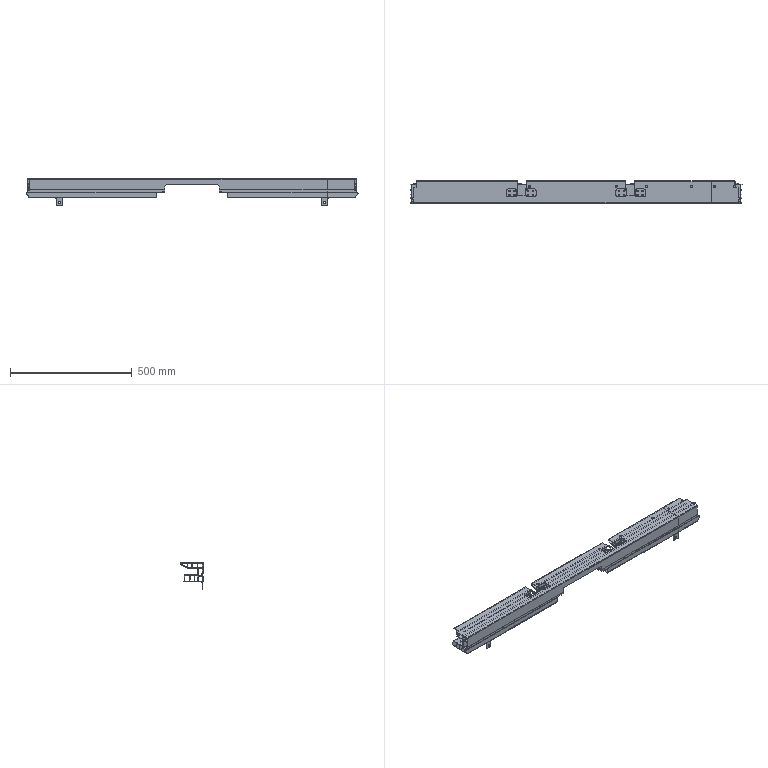NC program | NX | posted with a generic post | part box 1365 x 90.95 x 108.501 mm
Lines 36 to 1103 of 25066:
(CAVITY_MILL_1 , TOOL : D16)
N64 T16 M6
N66 G54
N68 G17 G0 G90 X693.761 Y-28.858 B0. C0. S9500 M3
N70 G43 Z30. H16
N72 Z0.527
N74 G94 G1 Z-0.973 F1000.
N76 X683.861 Y-34.573
N78 G3 X683.361 Y-35.439 R1.
N80 G1 X676.161
N82 Y-31.805 F2500.
N84 G2 X672.3 Y-33.633 R15.3
N86 G1 Y-39.073
N88 X676.161
N90 Y-35.439
N92 X683.361
N94 Y17.129
N96 G3 X684.77 Y22.775 R12.02
N98 G1 Y24.556
N100 G3 X683.361 Y30.203 R12.02
N102 G1 Y45.471
N104 G3 X682.561 Y46.273 R0.802
N106 G1 X677.738
N108 G3 X673.784 Y53.473 R10.019
N110 G1 X669.02
N112 G2 X675.85 Y45.473 R8.099
N114 G1 Y34.505
N116 X675.963 Y34.436
N118 X678.059 Y33.148
N120 G2 X682.85 Y24.556 R10.1
N122 G1 Y22.775
N124 G2 X675.85 Y13.163 R10.1
N126 G1 Y-19.025
N128 G2 X667.75 Y-27.125 R8.1
N130 G1 X665.1
N132 Y-45.473
N134 G2 X658.27 Y-53.473 R8.1
N136 G1 X663.033
N138 G3 X666.988 Y-46.273 R10.02
N140 G1 X682.561
N142 G3 X683.361 Y-45.473 R0.8
N144 G1 Y-35.439
N146 G2 X683.861 Y-34.573 R1.
N148 G1 X693.761 Y-28.858
N150 Z0.527
N152 G0 Z-0.444
N154 G1 Z-1.944 F1000.
N156 X683.861 Y-34.574
N158 G3 X683.361 Y-35.44 R1.
N160 G1 X676.161
N162 Y-31.805 F2500.
N164 G2 X672.3 Y-33.633 R15.3
N166 G1 Y-39.075
N168 X676.161
N170 Y-35.44
N172 X683.361
N174 Y17.129
N176 G3 X684.77 Y22.775 R12.02
N178 G1 Y24.556
N180 G3 X683.361 Y30.203 R12.02
N182 G1 Y45.475
N184 G3 X682.561 Y46.275 R0.8
N186 G1 X677.738
N188 G3 X673.783 Y53.475 R10.02
N190 G1 X669.019
N192 G2 X675.85 Y45.475 R8.1
N194 G1 Y34.505
N196 X675.933 Y34.455
N198 X678.059 Y33.148
N200 G2 X682.85 Y24.556 R10.1
N202 G1 Y22.775
N204 G2 X675.85 Y13.163 R10.1
N206 G1 Y-19.025
N208 G2 X667.75 Y-27.125 R8.1
N210 G1 X665.1
N212 Y-45.475
N214 G2 X658.269 Y-53.475 R8.1
N216 G1 X663.033
N218 G3 X666.988 Y-46.275 R10.02
N220 G1 X682.561
N222 G3 X683.361 Y-45.475 R0.8
N224 G1 Y-35.44
N226 G2 X683.861 Y-34.574 R1.
N228 G1 X693.761 Y-28.858
N230 Z-0.444
N232 G0 Z-1.416
N234 G1 Z-2.916 F1000.
N236 X683.861 Y-34.574
N238 G3 X683.361 Y-35.44 R1.
N240 G1 X676.161
N242 Y-31.805 F2500.
N244 G2 X672.3 Y-33.633 R15.3
N246 G1 Y-39.075
N248 X676.161
N250 Y-35.44
N252 X683.361
N254 Y17.129
N256 G3 X684.77 Y22.775 R12.02
N258 G1 Y24.556
N260 G3 X683.361 Y30.203 R12.02
N262 G1 Y45.475
N264 G3 X682.561 Y46.275 R0.8
N266 G1 X677.738
N268 G3 X673.783 Y53.475 R10.02
N270 G1 X669.019
N272 G2 X675.85 Y45.475 R8.1
N274 G1 Y34.505
N276 X675.963 Y34.436
N278 X678.059 Y33.148
N280 G2 X682.85 Y24.556 R10.1
N282 G1 Y22.775
N284 G2 X675.85 Y13.163 R10.1
N286 G1 Y-19.025
N288 G2 X667.75 Y-27.125 R8.1
N290 G1 X665.1
N292 Y-45.475
N294 G2 X658.269 Y-53.475 R8.1
N296 G1 X663.033
N298 G3 X666.988 Y-46.275 R10.02
N300 G1 X682.561
N302 G3 X683.361 Y-45.475 R0.8
N304 G1 Y-35.44
N306 G2 X683.861 Y-34.574 R1.
N308 G1 X693.761 Y-28.858
N310 Z-1.416
N312 G0 Z-2.387
N314 G1 Z-3.887 F1000.
N316 X683.861 Y-34.574
N318 G3 X683.361 Y-35.44 R1.
N320 G1 X676.161
N322 Y-31.805 F2500.
N324 G2 X672.3 Y-33.633 R15.3
N326 G1 Y-39.075
N328 X676.161
N330 Y-35.44
N332 X683.361
N334 Y17.129
N336 G3 X684.77 Y22.775 R12.02
N338 G1 Y24.556
N340 G3 X683.361 Y30.203 R12.02
N342 G1 Y45.475
N344 G3 X682.561 Y46.275 R0.8
N346 G1 X677.738
N348 G3 X673.783 Y53.475 R10.02
N350 G1 X669.019
N352 G2 X675.85 Y45.475 R8.1
N354 G1 Y34.505
N356 X675.963 Y34.436
N358 X678.059 Y33.148
N360 G2 X682.85 Y24.556 R10.1
N362 G1 Y22.775
N364 G2 X675.85 Y13.163 R10.1
N366 G1 Y-19.025
N368 G2 X667.75 Y-27.125 R8.1
N370 G1 X665.1
N372 Y-45.475
N374 G2 X658.269 Y-53.475 R8.1
N376 G1 X663.033
N378 G3 X666.988 Y-46.275 R10.02
N380 G1 X682.561
N382 G3 X683.361 Y-45.475 R0.8
N384 G1 Y-35.44
N386 G2 X683.861 Y-34.574 R1.
N388 G1 X693.761 Y-28.858
N390 Z-2.387
N392 G0 Z-3.358
N394 G1 Z-4.858 F1000.
N396 X683.861 Y-34.574
N398 G3 X683.361 Y-35.44 R1.
N400 G1 X676.161
N402 Y-31.805 F2500.
N404 G2 X672.3 Y-33.633 R15.3
N406 G1 Y-39.075
N408 X676.161
N410 Y-35.44
N412 X683.361
N414 Y17.129
N416 G3 X684.77 Y22.775 R12.02
N418 G1 Y24.556
N420 G3 X683.361 Y30.203 R12.02
N422 G1 Y45.475
N424 G3 X682.561 Y46.275 R0.8
N426 G1 X677.738
N428 G3 X673.783 Y53.475 R10.02
N430 G1 X669.019
N432 G2 X675.85 Y45.475 R8.1
N434 G1 Y34.505
N436 X675.963 Y34.436
N438 X678.059 Y33.148
N440 G2 X682.85 Y24.556 R10.1
N442 G1 Y22.775
N444 G2 X675.85 Y13.163 R10.1
N446 G1 Y-19.025
N448 G2 X667.75 Y-27.125 R8.1
N450 G1 X665.1
N452 Y-45.475
N454 G2 X658.269 Y-53.475 R8.1
N456 G1 X663.033
N458 G3 X666.988 Y-46.275 R10.02
N460 G1 X682.561
N462 G3 X683.361 Y-45.475 R0.8
N464 G1 Y-35.44
N466 G2 X683.861 Y-34.574 R1.
N468 G1 X693.761 Y-28.858
N470 Z-3.358
N472 G0 Z-4.33
N474 G1 Z-5.83 F1000.
N476 X683.861 Y-34.574
N478 G3 X683.361 Y-35.44 R1.
N480 G1 X676.161
N482 Y-31.805 F2500.
N484 G2 X672.3 Y-33.633 R15.3
N486 G1 Y-39.075
N488 X676.161
N490 Y-35.44
N492 X683.361
N494 Y17.129
N496 G3 X684.77 Y22.775 R12.02
N498 G1 Y24.556
N500 G3 X683.361 Y30.203 R12.02
N502 G1 Y45.475
N504 G3 X682.561 Y46.275 R0.8
N506 G1 X677.738
N508 G3 X673.783 Y53.475 R10.02
N510 G1 X669.019
N512 G2 X675.85 Y45.475 R8.1
N514 G1 Y34.505
N516 X678.059 Y33.148
N518 G2 X682.85 Y24.556 R10.1
N520 G1 Y22.775
N522 G2 X675.85 Y13.163 R10.1
N524 G1 Y-19.025
N526 G2 X667.75 Y-27.125 R8.1
N528 G1 X665.1
N530 Y-45.475
N532 G2 X658.269 Y-53.475 R8.1
N534 G1 X663.033
N536 G3 X666.988 Y-46.275 R10.02
N538 G1 X682.561
N540 G3 X683.361 Y-45.475 R0.8
N542 G1 Y-35.44
N544 G2 X683.861 Y-34.574 R1.
N546 G1 X693.761 Y-28.858
N548 Z-4.33
N550 G0 Z-5.301
N552 G1 Z-6.801 F1000.
N554 X683.861 Y-34.574
N556 G3 X683.361 Y-35.44 R1.
N558 G1 X676.161
N560 Y-31.805 F2500.
N562 G2 X672.3 Y-33.633 R15.3
N564 G1 Y-39.075
N566 X676.161
N568 Y-35.44
N570 X683.361
N572 Y17.129
N574 G3 X684.77 Y22.775 R12.02
N576 G1 Y24.556
N578 G3 X683.361 Y30.203 R12.02
N580 G1 Y45.475
N582 G3 X682.561 Y46.275 R0.8
N584 G1 X677.738
N586 G3 X673.783 Y53.475 R10.02
N588 G1 X669.019
N590 G2 X675.85 Y45.475 R8.1
N592 G1 Y34.505
N594 X678.059 Y33.148
N596 G2 X682.85 Y24.556 R10.1
N598 G1 Y22.775
N600 G2 X675.85 Y13.163 R10.1
N602 G1 Y-19.025
N604 G2 X667.75 Y-27.125 R8.1
N606 G1 X665.1
N608 Y-45.475
N610 G2 X658.269 Y-53.475 R8.1
N612 G1 X663.033
N614 G3 X666.988 Y-46.275 R10.02
N616 G1 X682.561
N618 G3 X683.361 Y-45.475 R0.8
N620 G1 Y-35.44
N622 G2 X683.861 Y-34.574 R1.
N624 G1 X693.761 Y-28.858
N626 Z-5.301
N628 G0 Z-6.273
N630 G1 Z-7.773 F1000.
N632 X683.861 Y-34.574
N634 G3 X683.361 Y-35.44 R1.
N636 G1 X676.161
N638 Y-31.805 F2500.
N640 G2 X672.3 Y-33.633 R15.3
N642 G1 Y-39.075
N644 X676.161
N646 Y-35.44
N648 X683.361
N650 Y17.129
N652 G3 X684.77 Y22.775 R12.02
N654 G1 Y24.556
N656 G3 X683.361 Y30.203 R12.02
N658 G1 Y45.475
N660 G3 X682.561 Y46.275 R0.8
N662 G1 X677.738
N664 G3 X673.783 Y53.475 R10.02
N666 G1 X669.019
N668 G2 X675.85 Y45.475 R8.1
N670 G1 Y34.505
N672 X678.059 Y33.148
N674 G2 X682.85 Y24.556 R10.1
N676 G1 Y22.775
N678 G2 X675.85 Y13.163 R10.1
N680 G1 Y-19.025
N682 G2 X667.75 Y-27.125 R8.1
N684 G1 X665.1
N686 Y-45.475
N688 G2 X658.269 Y-53.475 R8.1
N690 G1 X663.033
N692 G3 X666.988 Y-46.275 R10.02
N694 G1 X682.561
N696 G3 X683.361 Y-45.475 R0.8
N698 G1 Y-35.44
N700 G2 X683.861 Y-34.574 R1.
N702 G1 X693.761 Y-28.858
N704 Z-6.273
N706 G0 Z-7.244
N708 G1 Z-8.744 F1000.
N710 X683.861 Y-34.574
N712 G3 X683.361 Y-35.44 R1.
N714 G1 X676.161
N716 Y-31.805 F2500.
N718 G2 X672.3 Y-33.633 R15.3
N720 G1 Y-39.075
N722 X676.161
N724 Y-35.44
N726 X683.361
N728 Y17.129
N730 G3 X684.77 Y22.775 R12.02
N732 G1 Y24.556
N734 G3 X683.361 Y30.203 R12.02
N736 G1 Y45.475
N738 G3 X682.561 Y46.275 R0.8
N740 G1 X677.738
N742 G3 X673.783 Y53.475 R10.02
N744 G1 X669.019
N746 G2 X675.85 Y45.475 R8.1
N748 G1 Y34.505
N750 X678.059 Y33.148
N752 G2 X682.85 Y24.556 R10.1
N754 G1 Y22.775
N756 G2 X675.85 Y13.163 R10.1
N758 G1 Y-19.025
N760 G2 X667.75 Y-27.125 R8.1
N762 G1 X665.1
N764 Y-45.475
N766 G2 X658.269 Y-53.475 R8.1
N768 G1 X663.033
N770 G3 X666.988 Y-46.275 R10.02
N772 G1 X682.561
N774 G3 X683.361 Y-45.475 R0.8
N776 G1 Y-35.44
N778 G2 X683.861 Y-34.574 R1.
N780 G1 X693.761 Y-28.858
N782 Z-7.244
N784 G0 Z-8.216
N786 G1 Z-9.716 F1000.
N788 X683.861 Y-34.574
N790 G3 X683.361 Y-35.44 R1.
N792 G1 X676.161
N794 Y-31.805 F2500.
N796 G2 X672.3 Y-33.633 R15.3
N798 G1 Y-39.075
N800 X676.161
N802 Y-35.44
N804 X683.361
N806 Y17.129
N808 G3 X684.77 Y22.775 R12.02
N810 G1 Y24.556
N812 G3 X683.361 Y30.203 R12.02
N814 G1 Y45.475
N816 G3 X682.561 Y46.275 R0.8
N818 G1 X677.738
N820 G3 X673.783 Y53.475 R10.02
N822 G1 X669.019
N824 G2 X675.85 Y45.475 R8.1
N826 G1 Y34.505
N828 X678.059 Y33.149
N830 G2 X682.85 Y24.556 R10.1
N832 G1 Y22.775
N834 G2 X675.85 Y13.163 R10.1
N836 G1 Y-19.025
N838 G2 X667.75 Y-27.125 R8.1
N840 G1 X665.1
N842 Y-45.475
N844 G2 X658.269 Y-53.475 R8.1
N846 G1 X663.033
N848 G3 X666.988 Y-46.275 R10.02
N850 G1 X682.561
N852 G3 X683.361 Y-45.475 R0.8
N854 G1 Y-35.44
N856 G2 X683.861 Y-34.574 R1.
N858 G1 X693.761 Y-28.858
N860 Z-8.216
N862 G0 Z-9.187
N864 G1 Z-10.687 F1000.
N866 X683.861 Y-34.574
N868 G3 X683.361 Y-35.44 R1.
N870 G1 X676.161
N872 Y-31.805 F2500.
N874 G2 X672.3 Y-33.633 R15.3
N876 G1 Y-39.075
N878 X676.161
N880 Y-35.44
N882 X683.361
N884 Y17.129
N886 G3 X684.77 Y22.775 R12.02
N888 G1 Y24.556
N890 G3 X683.361 Y30.203 R12.02
N892 G1 Y45.475
N894 G3 X682.561 Y46.275 R0.8
N896 G1 X677.738
N898 G3 X673.783 Y53.475 R10.02
N900 G1 X669.019
N902 G2 X675.85 Y45.475 R8.1
N904 G1 Y34.505
N906 X678.037 Y33.162
N908 G2 X682.85 Y24.556 R10.1
N910 G1 Y22.775
N912 G2 X675.85 Y13.163 R10.1
N914 G1 Y-19.025
N916 G2 X667.75 Y-27.125 R8.1
N918 G1 X665.1
N920 Y-45.475
N922 G2 X658.269 Y-53.475 R8.1
N924 G1 X663.033
N926 G3 X666.988 Y-46.275 R10.02
N928 G1 X682.561
N930 G3 X683.361 Y-45.475 R0.8
N932 G1 Y-35.44
N934 G2 X683.861 Y-34.574 R1.
N936 G1 X693.761 Y-28.858
N938 Z-9.187
N940 G0 Z-10.158
N942 G1 Z-11.658 F1000.
N944 X683.861 Y-34.574
N946 G3 X683.361 Y-35.44 R1.
N948 G1 X676.161
N950 Y-31.805 F2500.
N952 G2 X672.3 Y-33.633 R15.3
N954 G1 Y-39.075
N956 X676.161
N958 Y-35.44
N960 X683.361
N962 Y17.129
N964 G3 X684.77 Y22.775 R12.02
N966 G1 Y24.556
N968 G3 X683.361 Y30.203 R12.02
N970 G1 Y45.475
N972 G3 X682.561 Y46.275 R0.8
N974 G1 X677.738
N976 G3 X673.783 Y53.475 R10.02
N978 G1 X669.019
N980 G2 X675.85 Y45.475 R8.1
N982 G1 Y34.505
N984 X678.037 Y33.162
N986 G2 X682.85 Y24.556 R10.1
N988 G1 Y22.775
N990 G2 X675.85 Y13.163 R10.1
N992 G1 Y-19.025
N994 G2 X667.75 Y-27.125 R8.1
N996 G1 X665.1
N998 Y-45.475
N1000 G2 X658.269 Y-53.475 R8.1
N1002 G1 X663.033
N1004 G3 X666.988 Y-46.275 R10.02
N1006 G1 X682.561
N1008 G3 X683.361 Y-45.475 R0.8
N1010 G1 Y-35.44
N1012 G2 X683.861 Y-34.574 R1.
N1014 G1 X693.761 Y-28.858
N1016 Z-10.158
N1018 G0 Z-11.13
N1020 G1 Z-12.63 F1000.
N1022 X683.861 Y-34.574
N1024 G3 X683.361 Y-35.44 R1.
N1026 G1 X676.161
N1028 Y-31.805 F2500.
N1030 G2 X672.3 Y-33.633 R15.3
N1032 G1 Y-39.075
N1034 X676.161
N1036 Y-35.44
N1038 X683.361
N1040 Y17.129
N1042 G3 X684.77 Y22.775 R12.02
N1044 G1 Y24.556
N1046 G3 X683.361 Y30.203 R12.02
N1048 G1 Y45.475
N1050 G3 X682.561 Y46.275 R0.8
N1052 G1 X677.738
N1054 G3 X673.783 Y53.475 R10.02
N1056 G1 X669.019
N1058 G2 X675.85 Y45.475 R8.1
N1060 G1 Y34.505
N1062 X678.037 Y33.162
N1064 G2 X682.85 Y24.556 R10.1
N1066 G1 Y22.775
N1068 G2 X675.85 Y13.163 R10.1
N1070 G1 Y-19.025
N1072 G2 X667.75 Y-27.125 R8.1
N1074 G1 X665.1
N1076 Y-45.475
N1078 G2 X658.269 Y-53.475 R8.1
N1080 G1 X663.033
N1082 G3 X666.988 Y-46.275 R10.02
N1084 G1 X682.561
N1086 G3 X683.361 Y-45.475 R0.8
N1088 G1 Y-35.44
N1090 G2 X683.861 Y-34.574 R1.
N1092 G1 X693.761 Y-28.858
N1094 Z-11.13
N1096 G0 Z-12.101
N1098 G1 Z-13.601 F1000.
N1100 X683.861 Y-34.574
N1102 G3 X683.361 Y-35.44 R1.
N1104 G1 X676.161
N1106 Y-31.805 F2500.
N1108 G2 X672.3 Y-33.633 R15.3
N1110 G1 Y-39.075
N1112 X676.161
N1114 Y-35.44
N1116 X683.361
N1118 Y17.129
N1120 G3 X684.77 Y22.775 R12.02
N1122 G1 Y24.556
N1124 G3 X683.361 Y30.203 R12.02
N1126 G1 Y45.475
N1128 G3 X682.561 Y46.275 R0.8
N1130 G1 X677.738
N1132 G3 X673.783 Y53.475 R10.02
N1134 G1 X669.019
N1136 G2 X675.85 Y45.475 R8.1
N1138 G1 Y34.505
N1140 X678.037 Y33.162
N1142 G2 X682.85 Y24.556 R10.1
N1144 G1 Y22.775
N1146 G2 X675.85 Y13.163 R10.1
N1148 G1 Y-19.025
N1150 G2 X667.75 Y-27.125 R8.1
N1152 G1 X665.1
N1154 Y-45.475
N1156 G2 X658.269 Y-53.475 R8.1
N1158 G1 X663.033
N1160 G3 X666.988 Y-46.275 R10.02
N1162 G1 X682.561
N1164 G3 X683.361 Y-45.475 R0.8
N1166 G1 Y-35.44
N1168 G2 X683.861 Y-34.574 R1.
N1170 G1 X693.761 Y-28.858
N1172 Z-12.101
N1174 G0 Z-13.073
N1176 G1 Z-14.573 F1000.
N1178 X683.861 Y-34.574
N1180 G3 X683.361 Y-35.44 R1.
N1182 G1 X676.161
N1184 Y-31.805 F2500.
N1186 G2 X672.3 Y-33.633 R15.3
N1188 G1 Y-39.075
N1190 X676.161
N1192 Y-35.44
N1194 X683.361
N1196 Y17.129
N1198 G3 X684.77 Y22.775 R12.02
N1200 G1 Y24.556
N1202 G3 X683.361 Y30.203 R12.02
N1204 G1 Y45.475
N1206 G3 X682.561 Y46.275 R0.8
N1208 G1 X677.738
N1210 G3 X673.783 Y53.475 R10.02
N1212 G1 X669.019
N1214 G2 X675.85 Y45.475 R8.1
N1216 G1 Y34.505
N1218 X678.037 Y33.162
N1220 G2 X682.85 Y24.556 R10.1
N1222 G1 Y22.775
N1224 G2 X675.85 Y13.163 R10.1
N1226 G1 Y-19.025
N1228 G2 X667.75 Y-27.125 R8.1
N1230 G1 X665.1
N1232 Y-45.475
N1234 G2 X658.269 Y-53.475 R8.1
N1236 G1 X663.033
N1238 G3 X666.988 Y-46.275 R10.02
N1240 G1 X682.561
N1242 G3 X683.361 Y-45.475 R0.8
N1244 G1 Y-35.44
N1246 G2 X683.861 Y-34.574 R1.
N1248 G1 X693.761 Y-28.858
N1250 Z-13.073
N1252 G0 Z-14.044
N1254 G1 Z-15.544 F1000.
N1256 X683.861 Y-34.574
N1258 G3 X683.361 Y-35.44 R1.
N1260 G1 X676.161
N1262 Y-31.805 F2500.
N1264 G2 X672.3 Y-33.633 R15.3
N1266 G1 Y-39.075
N1268 X676.161
N1270 Y-35.44
N1272 X683.361
N1274 Y17.129
N1276 G3 X684.77 Y22.775 R12.02
N1278 G1 Y24.556
N1280 G3 X683.361 Y30.203 R12.02
N1282 G1 Y45.475
N1284 G3 X682.561 Y46.275 R0.8
N1286 G1 X677.738
N1288 G3 X673.783 Y53.475 R10.02
N1290 G1 X669.019
N1292 G2 X675.85 Y45.475 R8.1
N1294 G1 Y34.505
N1296 X678.037 Y33.162
N1298 G2 X682.85 Y24.556 R10.1
N1300 G1 Y22.775
N1302 G2 X675.85 Y13.163 R10.1
N1304 G1 Y-19.025
N1306 G2 X667.75 Y-27.125 R8.1
N1308 G1 X665.1
N1310 Y-45.475
N1312 G2 X658.269 Y-53.475 R8.1
N1314 G1 X663.033
N1316 G3 X666.988 Y-46.275 R10.02
N1318 G1 X682.561
N1320 G3 X683.361 Y-45.475 R0.8
N1322 G1 Y-35.44
N1324 G2 X683.861 Y-34.574 R1.
N1326 G1 X693.761 Y-28.858
N1328 Z-14.044
N1330 G0 Z-15.016
N1332 G1 Z-16.516 F1000.
N1334 X683.861 Y-34.574
N1336 G3 X683.361 Y-35.44 R1.
N1338 G1 X676.161
N1340 Y-31.805 F2500.
N1342 G2 X672.3 Y-33.633 R15.3
N1344 G1 Y-39.075
N1346 X676.161
N1348 Y-35.44
N1350 X683.361
N1352 Y17.129
N1354 G3 X684.77 Y22.775 R12.02
N1356 G1 Y24.556
N1358 G3 X683.361 Y30.203 R12.02
N1360 G1 Y45.475
N1362 G3 X682.561 Y46.275 R0.8
N1364 G1 X677.738
N1366 G3 X673.783 Y53.475 R10.02
N1368 G1 X669.019
N1370 G2 X675.85 Y45.475 R8.1
N1372 G1 Y34.505
N1374 X678.037 Y33.162
N1376 G2 X682.85 Y24.556 R10.1
N1378 G1 Y22.775
N1380 G2 X675.85 Y13.163 R10.1
N1382 G1 Y-19.025
N1384 G2 X667.75 Y-27.125 R8.1
N1386 G1 X665.1
N1388 Y-45.475
N1390 G2 X658.269 Y-53.475 R8.1
N1392 G1 X663.033
N1394 G3 X666.988 Y-46.275 R10.02
N1396 G1 X682.561
N1398 G3 X683.361 Y-45.475 R0.8
N1400 G1 Y-35.44
N1402 G2 X683.861 Y-34.574 R1.
N1404 G1 X693.761 Y-28.858
N1406 Z-15.016
N1408 G0 Z-15.987
N1410 G1 Z-17.487 F1000.
N1412 X683.861 Y-34.574
N1414 G3 X683.361 Y-35.44 R1.
N1416 G1 X676.161
N1418 Y-31.805 F2500.
N1420 G2 X672.3 Y-33.633 R15.3
N1422 G1 Y-39.075
N1424 X676.161
N1426 Y-35.44
N1428 X683.361
N1430 Y17.129
N1432 G3 X684.77 Y22.775 R12.02
N1434 G1 Y24.556
N1436 G3 X683.361 Y30.203 R12.02
N1438 G1 Y45.475
N1440 G3 X682.561 Y46.275 R0.8
N1442 G1 X677.738
N1444 G3 X673.783 Y53.475 R10.02
N1446 G1 X669.019
N1448 G2 X675.85 Y45.475 R8.1
N1450 G1 Y34.505
N1452 X678.037 Y33.162
N1454 G2 X682.85 Y24.556 R10.1
N1456 G1 Y22.775
N1458 G2 X675.85 Y13.163 R10.1
N1460 G1 Y-19.025
N1462 G2 X667.75 Y-27.125 R8.1
N1464 G1 X665.1
N1466 Y-45.475
N1468 G2 X658.269 Y-53.475 R8.1
N1470 G1 X663.033
N1472 G3 X666.988 Y-46.275 R10.02
N1474 G1 X682.561
N1476 G3 X683.361 Y-45.475 R0.8
N1478 G1 Y-35.44
N1480 G2 X683.861 Y-34.574 R1.
N1482 G1 X693.761 Y-28.858
N1484 Z-15.987
N1486 G0 Z-16.958
N1488 G1 Z-18.458 F1000.
N1490 X683.861 Y-34.574
N1492 G3 X683.361 Y-35.44 R1.
N1494 G1 X676.161
N1496 Y-31.805 F2500.
N1498 G2 X672.3 Y-33.633 R15.3
N1500 G1 Y-39.075
N1502 X676.161
N1504 Y-35.44
N1506 X683.361
N1508 Y17.129
N1510 G3 X684.77 Y22.775 R12.02
N1512 G1 Y24.556
N1514 G3 X683.361 Y30.203 R12.02
N1516 G1 Y45.475
N1518 G3 X682.561 Y46.275 R0.8
N1520 G1 X677.738
N1522 G3 X673.783 Y53.475 R10.02
N1524 G1 X669.019
N1526 G2 X675.85 Y45.475 R8.1
N1528 G1 Y34.505
N1530 X678.037 Y33.162
N1532 G2 X682.85 Y24.556 R10.1
N1534 G1 Y22.775
N1536 G2 X675.85 Y13.163 R10.1
N1538 G1 Y-19.025
N1540 G2 X667.75 Y-27.125 R8.1
N1542 G1 X665.1
N1544 Y-45.475
N1546 G2 X658.269 Y-53.475 R8.1
N1548 G1 X663.033
N1550 G3 X666.988 Y-46.275 R10.02
N1552 G1 X682.561
N1554 G3 X683.361 Y-45.475 R0.8
N1556 G1 Y-35.44
N1558 G2 X683.861 Y-34.574 R1.
N1560 G1 X693.761 Y-28.858
N1562 Z-16.958
N1564 G0 Z-17.93
N1566 G1 Z-19.43 F1000.
N1568 X683.861 Y-34.574
N1570 G3 X683.361 Y-35.44 R1.
N1572 G1 X676.161
N1574 Y-31.805 F2500.
N1576 G2 X672.3 Y-33.633 R15.3
N1578 G1 Y-39.075
N1580 X676.161
N1582 Y-35.44
N1584 X683.361
N1586 Y17.129
N1588 G3 X684.77 Y22.775 R12.02
N1590 G1 Y24.556
N1592 G3 X683.361 Y30.203 R12.02
N1594 G1 Y45.475
N1596 G3 X682.561 Y46.275 R0.8
N1598 G1 X677.738
N1600 G3 X673.783 Y53.475 R10.02
N1602 G1 X669.019
N1604 G2 X675.85 Y45.475 R8.1
N1606 G1 Y34.505
N1608 X678.037 Y33.162
N1610 G2 X682.85 Y24.556 R10.1
N1612 G1 Y22.775
N1614 G2 X675.85 Y13.163 R10.1
N1616 G1 Y-19.025
N1618 G2 X667.75 Y-27.125 R8.1
N1620 G1 X665.1
N1622 Y-45.475
N1624 G2 X658.269 Y-53.475 R8.1
N1626 G1 X663.033
N1628 G3 X666.988 Y-46.275 R10.02
N1630 G1 X682.561
N1632 G3 X683.361 Y-45.475 R0.8
N1634 G1 Y-35.44
N1636 G2 X683.861 Y-34.574 R1.
N1638 G1 X693.761 Y-28.858
N1640 Z-17.93
N1642 G0 Z-18.901
N1644 G1 Z-20.401 F1000.
N1646 X683.861 Y-34.574
N1648 G3 X683.361 Y-35.44 R1.
N1650 G1 X676.161
N1652 Y-31.805 F2500.
N1654 G2 X672.3 Y-33.633 R15.3
N1656 G1 Y-39.075
N1658 X676.161
N1660 Y-35.44
N1662 X683.361
N1664 Y17.129
N1666 G3 X684.77 Y22.775 R12.02
N1668 G1 Y24.556
N1670 G3 X683.361 Y30.203 R12.02
N1672 G1 Y45.475
N1674 G3 X682.561 Y46.275 R0.8
N1676 G1 X677.738
N1678 G3 X673.783 Y53.475 R10.02
N1680 G1 X669.019
N1682 G2 X675.85 Y45.475 R8.1
N1684 G1 Y34.505
N1686 X678.037 Y33.162
N1688 G2 X682.85 Y24.556 R10.1
N1690 G1 Y22.775
N1692 G2 X675.85 Y13.163 R10.1
N1694 G1 Y-19.025
N1696 G2 X667.75 Y-27.125 R8.1
N1698 G1 X665.1
N1700 Y-45.475
N1702 G2 X658.269 Y-53.475 R8.1
N1704 G1 X663.033
N1706 G3 X666.988 Y-46.275 R10.02
N1708 G1 X682.561
N1710 G3 X683.361 Y-45.475 R0.8
N1712 G1 Y-35.44
N1714 G2 X683.861 Y-34.574 R1.
N1716 G1 X693.761 Y-28.858
N1718 Z-18.901
N1720 G0 Z-19.201
N1722 G1 Z-20.701 F1000.
N1724 X683.861 Y-34.574
N1726 G3 X683.361 Y-35.44 R1.
N1728 G1 X676.161
N1730 Y-31.805 F2500.
N1732 G2 X672.3 Y-33.633 R15.3
N1734 G1 Y-39.075
N1736 X676.161
N1738 Y-35.44
N1740 X683.361
N1742 Y17.129
N1744 G3 X684.77 Y22.775 R12.02
N1746 G1 Y24.556
N1748 G3 X683.361 Y30.203 R12.02
N1750 G1 Y45.475
N1752 G3 X682.561 Y46.275 R0.8
N1754 G1 X677.738
N1756 G3 X673.783 Y53.475 R10.02
N1758 G1 X669.019
N1760 G2 X675.85 Y45.475 R8.1
N1762 G1 Y34.505
N1764 X675.948 Y34.445
N1766 X678.037 Y33.162
N1768 G2 X682.85 Y24.556 R10.1
N1770 G1 Y22.775
N1772 G2 X675.85 Y13.163 R10.1
N1774 G1 Y-19.025
N1776 G2 X667.75 Y-27.125 R8.1
N1778 G1 X665.1
N1780 Y-45.475
N1782 G2 X658.269 Y-53.475 R8.1
N1784 G1 X663.033
N1786 G3 X666.988 Y-46.275 R10.02
N1788 G1 X682.561
N1790 G3 X683.361 Y-45.475 R0.8
N1792 G1 Y-35.44
N1794 G2 X683.861 Y-34.574 R1.
N1796 G1 X693.761 Y-28.858
N1798 Z-19.201
N1800 G0 Z-20.188
N1802 G1 Z-21.688 F1000.
N1804 X683.861 Y-34.574
N1806 G3 X683.361 Y-35.44 R1.
N1808 G1 X676.161
N1810 Y-31.805 F2500.
N1812 G2 X672.3 Y-33.633 R15.3
N1814 G1 Y-39.075
N1816 X676.161
N1818 Y-35.44
N1820 X683.361
N1822 Y17.129
N1824 G3 X684.77 Y22.775 R12.02
N1826 G1 Y24.556
N1828 G3 X683.361 Y30.203 R12.02
N1830 G1 Y45.475
N1832 G3 X682.561 Y46.275 R0.8
N1834 G1 X677.738
N1836 G3 X673.783 Y53.475 R10.02
N1838 G1 X669.019
N1840 G2 X675.85 Y45.475 R8.1
N1842 G1 Y34.505
N1844 X675.948 Y34.445
N1846 X678.037 Y33.162
N1848 G2 X682.85 Y24.556 R10.1
N1850 G1 Y22.775
N1852 G2 X675.85 Y13.163 R10.1
N1854 G1 Y-19.025
N1856 G2 X667.75 Y-27.125 R8.1
N1858 G1 X665.1
N1860 Y-45.475
N1862 G2 X658.269 Y-53.475 R8.1
N1864 G1 X663.033
N1866 G3 X666.988 Y-46.275 R10.02
N1868 G1 X682.561
N1870 G3 X683.361 Y-45.475 R0.8
N1872 G1 Y-35.44
N1874 G2 X683.861 Y-34.574 R1.
N1876 G1 X693.761 Y-28.858
N1878 Z-20.188
N1880 G0 Z-21.175
N1882 G1 Z-22.675 F1000.
N1884 X683.861 Y-34.574
N1886 G3 X683.361 Y-35.44 R1.
N1888 G1 X676.161
N1890 Y-31.805 F2500.
N1892 G2 X672.3 Y-33.633 R15.3
N1894 G1 Y-39.075
N1896 X676.161
N1898 Y-35.44
N1900 X683.361
N1902 Y17.129
N1904 G3 X684.77 Y22.775 R12.02
N1906 G1 Y24.556
N1908 G3 X683.361 Y30.203 R12.02
N1910 G1 Y45.475
N1912 G3 X682.561 Y46.275 R0.8
N1914 G1 X677.738
N1916 G3 X673.783 Y53.475 R10.02
N1918 G1 X669.019
N1920 G2 X675.85 Y45.475 R8.1
N1922 G1 Y34.505
N1924 X675.948 Y34.445
N1926 X678.037 Y33.162
N1928 G2 X682.85 Y24.556 R10.1
N1930 G1 Y22.775
N1932 G2 X675.85 Y13.163 R10.1
N1934 G1 Y-19.025
N1936 G2 X667.75 Y-27.125 R8.1
N1938 G1 X665.1
N1940 Y-45.475
N1942 G2 X658.269 Y-53.475 R8.1
N1944 G1 X663.033
N1946 G3 X666.988 Y-46.275 R10.02
N1948 G1 X682.561
N1950 G3 X683.361 Y-45.475 R0.8
N1952 G1 Y-35.44
N1954 G2 X683.861 Y-34.574 R1.
N1956 G1 X693.761 Y-28.858
N1958 Z-21.175
N1960 G0 Z-22.162
N1962 G1 Z-23.662 F1000.
N1964 X683.861 Y-34.574
N1966 G3 X683.361 Y-35.44 R1.
N1968 G1 X676.161
N1970 Y-31.805 F2500.
N1972 G2 X672.3 Y-33.633 R15.3
N1974 G1 Y-39.075
N1976 X676.161
N1978 Y-35.44
N1980 X683.361
N1982 Y17.129
N1984 G3 X684.77 Y22.775 R12.02
N1986 G1 Y24.556
N1988 G3 X683.361 Y30.203 R12.02
N1990 G1 Y45.475
N1992 G3 X682.561 Y46.275 R0.8
N1994 G1 X677.738
N1996 G3 X673.783 Y53.475 R10.02
N1998 G1 X669.019
N2000 G2 X675.85 Y45.475 R8.1
N2002 G1 Y34.505
N2004 X675.948 Y34.445
N2006 X678.037 Y33.162
N2008 G2 X682.85 Y24.556 R10.1
N2010 G1 Y22.775
N2012 G2 X675.85 Y13.163 R10.1
N2014 G1 Y-19.025
N2016 G2 X667.75 Y-27.125 R8.1
N2018 G1 X665.1
N2020 Y-45.475
N2022 G2 X658.269 Y-53.475 R8.1
N2024 G1 X663.033
N2026 G3 X666.988 Y-46.275 R10.02
N2028 G1 X682.561
N2030 G3 X683.361 Y-45.475 R0.8
N2032 G1 Y-35.44
N2034 G2 X683.861 Y-34.574 R1.
N2036 G1 X693.761 Y-28.858
N2038 Z-22.162
N2040 G0 Z-23.149
N2042 G1 Z-24.649 F1000.
N2044 X683.861 Y-34.574
N2046 G3 X683.361 Y-35.44 R1.
N2048 G1 X676.161
N2050 Y-31.805 F2500.
N2052 G2 X672.3 Y-33.633 R15.3
N2054 G1 Y-39.075
N2056 X676.161
N2058 Y-35.44
N2060 X683.361
N2062 Y17.129
N2064 G3 X684.77 Y22.775 R12.02
N2066 G1 Y24.556
N2068 G3 X683.361 Y30.203 R12.02
N2070 G1 Y45.475
N2072 G3 X682.561 Y46.275 R0.8
N2074 G1 X677.738
N2076 G3 X673.783 Y53.475 R10.02
N2078 G1 X669.019
N2080 G2 X675.85 Y45.475 R8.1
N2082 G1 Y34.505
N2084 X675.948 Y34.445
N2086 X678.037 Y33.162
N2088 G2 X682.85 Y24.556 R10.1
N2090 G1 Y22.775
N2092 G2 X675.85 Y13.163 R10.1
N2094 G1 Y-19.025
N2096 G2 X667.75 Y-27.125 R8.1
N2098 G1 X665.1
N2100 Y-45.475
N2102 G2 X658.269 Y-53.475 R8.1
N2104 G1 X663.033
N2106 G3 X666.988 Y-46.275 R10.02
N2108 G1 X682.561
N2110 G3 X683.361 Y-45.475 R0.8
N2112 G1 Y-35.44
N2114 G2 X683.861 Y-34.574 R1.
N2116 G1 X693.761 Y-28.858
N2118 Z-23.149
N2120 G0 Z-24.136
N2122 G1 Z-25.636 F1000.
N2124 X683.861 Y-34.574
N2126 G3 X683.361 Y-35.44 R1.
N2128 G1 X676.161
N2130 Y-31.805 F2500.
N2132 G2 X672.3 Y-33.633 R15.3
N2134 G1 Y-39.075
N2136 X676.161
N2138 Y-35.44
N2140 X683.361
N2142 Y17.129
N2144 G3 X684.77 Y22.775 R12.02
N2146 G1 Y24.556
N2148 G3 X683.361 Y30.203 R12.02
N2150 G1 Y45.475
N2152 G3 X682.561 Y46.275 R0.8
N2154 G1 X677.738
N2156 G3 X673.783 Y53.475 R10.02
N2158 G1 X669.019
N2160 G2 X675.85 Y45.475 R8.1
N2162 G1 Y34.505
N2164 X675.948 Y34.445
N2166 X678.037 Y33.162
N2168 G2 X682.85 Y24.556 R10.1
N2170 G1 Y22.775
N2172 G2 X675.85 Y13.163 R10.1
N2174 G1 Y-19.025
N2176 G2 X667.75 Y-27.125 R8.1
N2178 G1 X665.1
N2180 Y-45.475
N2182 G2 X658.269 Y-53.475 R8.1
N2184 G1 X663.033
N2186 G3 X666.988 Y-46.275 R10.02
N2188 G1 X682.561
N2190 G3 X683.361 Y-45.475 R0.8
N2192 G1 Y-35.44